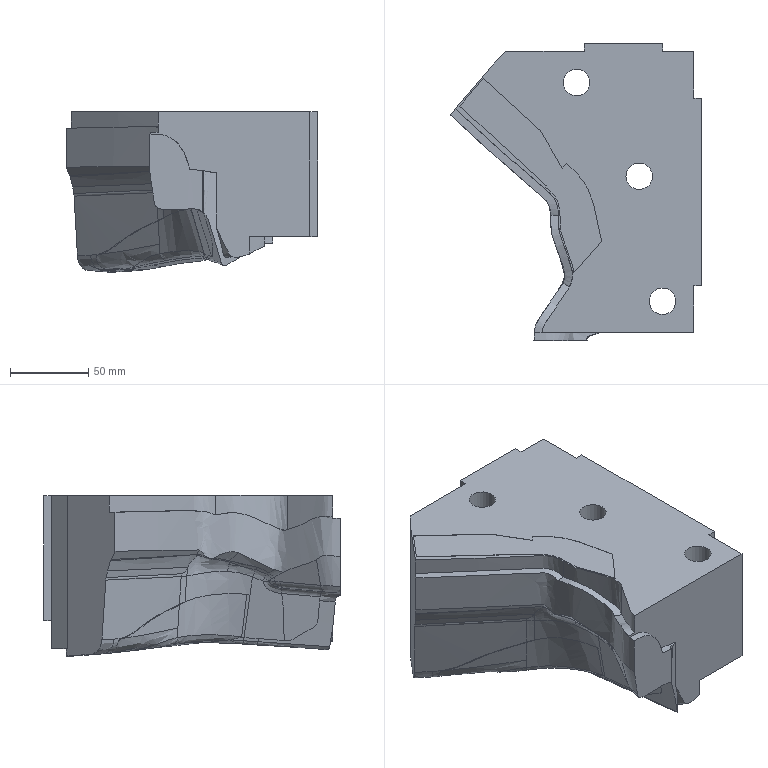Part | NX | features solid 2 | 1 solid | 126 faces | box 160.857 x 190.021 x 103.104 mm | volume 1615929 mm3 | spline 82 | plane 34 | cylinder 9 | sphere 1 | commonest cylinder face diameters 17 x3 25 x3 10 x2 60 x1